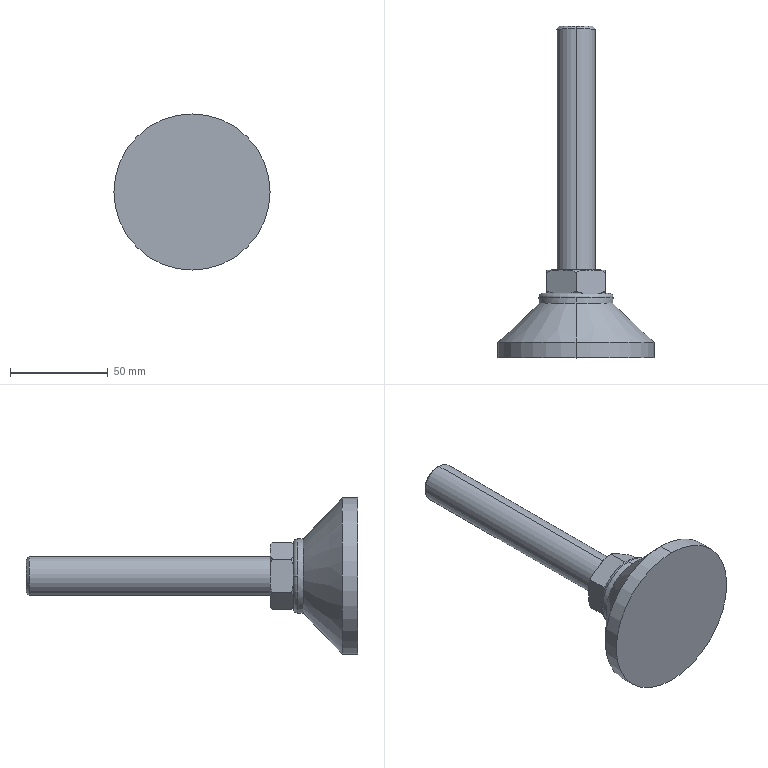Part | SolidWorks | features BaseBody 1 | 1 solid | 36 faces | box 80 x 170 x 80 mm | volume 151225 mm3 | torus 16 | plane 10 | cylinder 6 | cone 4 | commonest cylinder face diameters 20 x2 38 x2 80 x2